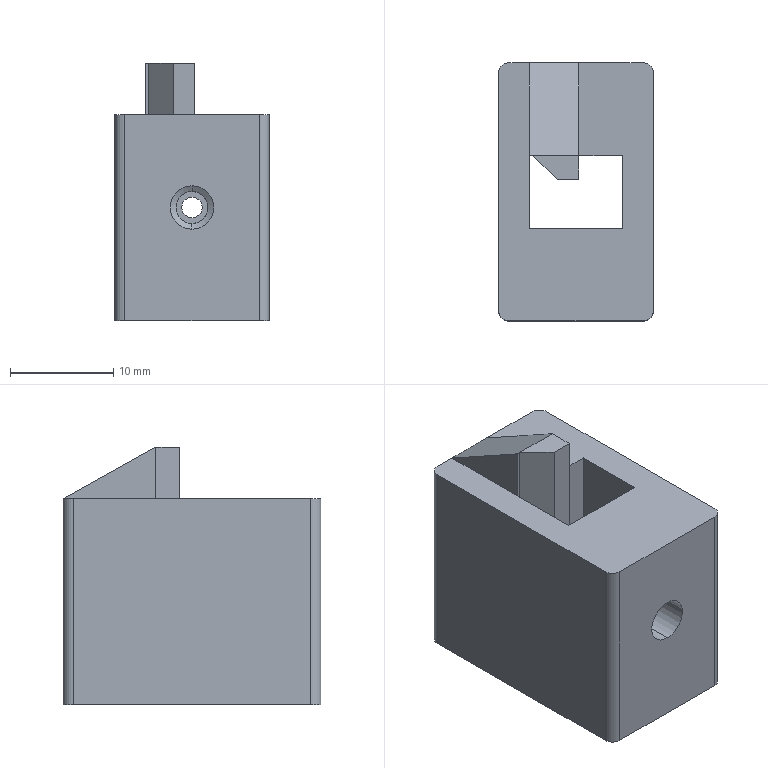Part | STEP file | 03-06 right pre-press cutter plate | 1 solid | 39 faces | box 15 x 25 x 25 mm | volume 5962 mm3 | plane 21 | cylinder 16 | cone 2 | commonest cylinder face diameters 2 x6 3.1 x4 7 x4 4.2 x2
STEP:
#1=CARTESIAN_POINT('',(0.,9.5,12.));
#2=VERTEX_POINT('',#1);
#3=CARTESIAN_POINT('',(0.,9.5,10.));
#4=VERTEX_POINT('',#3);
#5=CARTESIAN_POINT('',(0.,9.5,11.));
#6=DIRECTION('',(0.,-1.,0.));
#7=DIRECTION('',(0.,0.,-1.));
#8=AXIS2_PLACEMENT_3D('',#5,#6,#7);
#9=CIRCLE('',#8,1.);
#10=EDGE_CURVE('',#2,#4,#9,.T.);
#11=ORIENTED_EDGE('',*,*,#10,.T.);
#12=CARTESIAN_POINT('',(0.,12.5,10.));
#13=VERTEX_POINT('',#12);
#14=CARTESIAN_POINT('',(0.,2.5,10.));
#15=DIRECTION('',(0.,1.,0.));
#16=VECTOR('',#15,1000.);
#17=LINE('',#14,#16);
#18=EDGE_CURVE('',#4,#13,#17,.T.);
#19=ORIENTED_EDGE('',*,*,#18,.T.);
#20=CARTESIAN_POINT('',(0.,12.5,12.));
#21=VERTEX_POINT('',#20);
#22=CARTESIAN_POINT('',(0.,12.5,11.));
#23=DIRECTION('',(0.,1.,0.));
#24=DIRECTION('',(0.,0.,1.));
#25=AXIS2_PLACEMENT_3D('',#22,#23,#24);
#26=CIRCLE('',#25,1.);
#27=EDGE_CURVE('',#13,#21,#26,.T.);
#28=ORIENTED_EDGE('',*,*,#27,.T.);
#29=CARTESIAN_POINT('',(0.,2.5,12.));
#30=DIRECTION('',(0.,1.,0.));
#31=VECTOR('',#30,1000.);
#32=LINE('',#29,#31);
#33=EDGE_CURVE('',#2,#21,#32,.T.);
#34=ORIENTED_EDGE('',*,*,#33,.F.);
#35=EDGE_LOOP('',(#11,#19,#28,#34));
#36=FACE_OUTER_BOUND('',#35,.T.);
#37=CARTESIAN_POINT('',(0.,2.5,11.));
#38=DIRECTION('',(0.,1.,0.));
#39=DIRECTION('',(0.,0.,1.));
#40=AXIS2_PLACEMENT_3D('',#37,#38,#39);
#41=CYLINDRICAL_SURFACE('',#40,1.);
#42=ADVANCED_FACE('',(#36),#41,.F.);
#43=CARTESIAN_POINT('',(0.,-7.5,13.1));
#44=VERTEX_POINT('',#43);
#45=CARTESIAN_POINT('',(0.,-7.5,8.9));
#46=VERTEX_POINT('',#45);
#47=CARTESIAN_POINT('',(0.,-7.5,11.));
#48=DIRECTION('',(0.,-1.,0.));
#49=DIRECTION('',(0.,0.,-1.));
#50=AXIS2_PLACEMENT_3D('',#47,#48,#49);
#51=CIRCLE('',#50,2.1);
#52=EDGE_CURVE('',#44,#46,#51,.T.);
#53=ORIENTED_EDGE('',*,*,#52,.F.);
#54=CARTESIAN_POINT('',(0.,-12.5,13.1));
#55=VERTEX_POINT('',#54);
#56=CARTESIAN_POINT('',(0.,-12.5,13.1));
#57=DIRECTION('',(0.,-1.,0.));
#58=VECTOR('',#57,1000.);
#59=LINE('',#56,#58);
#60=EDGE_CURVE('',#44,#55,#59,.T.);
#61=ORIENTED_EDGE('',*,*,#60,.T.);
#62=CARTESIAN_POINT('',(0.,-12.5,8.9));
#63=VERTEX_POINT('',#62);
#64=CARTESIAN_POINT('',(0.,-12.5,11.));
#65=DIRECTION('',(0.,-1.,0.));
#66=DIRECTION('',(0.,0.,-1.));
#67=AXIS2_PLACEMENT_3D('',#64,#65,#66);
#68=CIRCLE('',#67,2.1);
#69=EDGE_CURVE('',#55,#63,#68,.T.);
#70=ORIENTED_EDGE('',*,*,#69,.T.);
#71=CARTESIAN_POINT('',(0.,-12.5,8.9));
#72=DIRECTION('',(0.,-1.,0.));
#73=VECTOR('',#72,1000.);
#74=LINE('',#71,#73);
#75=EDGE_CURVE('',#46,#63,#74,.T.);
#76=ORIENTED_EDGE('',*,*,#75,.F.);
#77=EDGE_LOOP('',(#53,#61,#70,#76));
#78=FACE_OUTER_BOUND('',#77,.T.);
#79=CARTESIAN_POINT('',(0.,-12.5,11.));
#80=DIRECTION('',(0.,-1.,0.));
#81=DIRECTION('',(0.,0.,-1.));
#82=AXIS2_PLACEMENT_3D('',#79,#80,#81);
#83=CYLINDRICAL_SURFACE('',#82,2.1);
#84=ADVANCED_FACE('',(#78),#83,.F.);
#85=CARTESIAN_POINT('',(0.,-7.17,12.55));
#86=VERTEX_POINT('',#85);
#87=CARTESIAN_POINT('',(0.,-7.17,9.45));
#88=VERTEX_POINT('',#87);
#89=CARTESIAN_POINT('',(0.,-7.17,11.));
#90=DIRECTION('',(0.,-1.,0.));
#91=DIRECTION('',(0.,0.,-1.));
#92=AXIS2_PLACEMENT_3D('',#89,#90,#91);
#93=CIRCLE('',#92,1.55);
#94=EDGE_CURVE('',#86,#88,#93,.T.);
#95=ORIENTED_EDGE('',*,*,#94,.F.);
#96=CARTESIAN_POINT('',(0.,-7.5,13.1));
#97=DIRECTION('',(0.,-0.515,0.8572));
#98=VECTOR('',#97,1000.);
#99=LINE('',#96,#98);
#100=EDGE_CURVE('',#86,#44,#99,.T.);
#101=ORIENTED_EDGE('',*,*,#100,.T.);
#102=ORIENTED_EDGE('',*,*,#52,.T.);
#103=CARTESIAN_POINT('',(0.,-7.5,8.9));
#104=DIRECTION('',(0.,-0.515,-0.8572));
#105=VECTOR('',#104,1000.);
#106=LINE('',#103,#105);
#107=EDGE_CURVE('',#88,#46,#106,.T.);
#108=ORIENTED_EDGE('',*,*,#107,.F.);
#109=EDGE_LOOP('',(#95,#101,#102,#108));
#110=FACE_OUTER_BOUND('',#109,.T.);
#111=CARTESIAN_POINT('',(0.,-7.5,11.));
#112=DIRECTION('',(0.,-1.,0.));
#113=DIRECTION('',(0.,0.,-1.));
#114=AXIS2_PLACEMENT_3D('',#111,#112,#113);
#115=CONICAL_SURFACE('',#114,2.1,1.03);
#116=ADVANCED_FACE('',(#110),#115,.F.);
#117=CARTESIAN_POINT('',(0.,-3.51,12.55));
#118=VERTEX_POINT('',#117);
#119=CARTESIAN_POINT('',(0.,-3.51,9.45));
#120=VERTEX_POINT('',#119);
#121=CARTESIAN_POINT('',(0.,-3.51,11.));
#122=DIRECTION('',(0.,-1.,0.));
#123=DIRECTION('',(1.,0.,0.));
#124=AXIS2_PLACEMENT_3D('',#121,#122,#123);
#125=CIRCLE('',#124,1.55);
#126=EDGE_CURVE('',#118,#120,#125,.T.);
#127=ORIENTED_EDGE('',*,*,#126,.F.);
#128=CARTESIAN_POINT('',(0.,9.5,12.55));
#129=DIRECTION('',(0.,-1.,0.));
#130=VECTOR('',#129,1000.);
#131=LINE('',#128,#130);
#132=EDGE_CURVE('',#118,#86,#131,.T.);
#133=ORIENTED_EDGE('',*,*,#132,.T.);
#134=ORIENTED_EDGE('',*,*,#94,.T.);
#135=CARTESIAN_POINT('',(0.,9.5,9.45));
#136=DIRECTION('',(0.,-1.,0.));
#137=VECTOR('',#136,1000.);
#138=LINE('',#135,#137);
#139=EDGE_CURVE('',#120,#88,#138,.T.);
#140=ORIENTED_EDGE('',*,*,#139,.F.);
#141=EDGE_LOOP('',(#127,#133,#134,#140));
#142=FACE_OUTER_BOUND('',#141,.T.);
#143=CARTESIAN_POINT('',(0.,9.5,11.));
#144=DIRECTION('',(0.,-1.,0.));
#145=DIRECTION('',(0.,0.,-1.));
#146=AXIS2_PLACEMENT_3D('',#143,#144,#145);
#147=CYLINDRICAL_SURFACE('',#146,1.55);
#148=ADVANCED_FACE('',(#142),#147,.F.);
#149=CARTESIAN_POINT('',(0.,9.5,12.55));
#150=VERTEX_POINT('',#149);
#151=CARTESIAN_POINT('',(0.,9.5,9.45));
#152=VERTEX_POINT('',#151);
#153=CARTESIAN_POINT('',(0.,9.5,11.));
#154=DIRECTION('',(0.,-1.,0.));
#155=DIRECTION('',(0.,0.,-1.));
#156=AXIS2_PLACEMENT_3D('',#153,#154,#155);
#157=CIRCLE('',#156,1.55);
#158=EDGE_CURVE('',#150,#152,#157,.T.);
#159=ORIENTED_EDGE('',*,*,#158,.F.);
#160=CARTESIAN_POINT('',(0.,1.199,12.55));
#161=VERTEX_POINT('',#160);
#162=CARTESIAN_POINT('',(0.,9.5,12.55));
#163=DIRECTION('',(0.,-1.,0.));
#164=VECTOR('',#163,1000.);
#165=LINE('',#162,#164);
#166=EDGE_CURVE('',#150,#161,#165,.T.);
#167=ORIENTED_EDGE('',*,*,#166,.T.);
#168=CARTESIAN_POINT('',(0.,1.199,9.45));
#169=VERTEX_POINT('',#168);
#170=CARTESIAN_POINT('',(0.,1.199,11.));
#171=DIRECTION('',(0.,1.,0.));
#172=DIRECTION('',(0.,0.,1.));
#173=AXIS2_PLACEMENT_3D('',#170,#171,#172);
#174=CIRCLE('',#173,1.55);
#175=EDGE_CURVE('',#169,#161,#174,.T.);
#176=ORIENTED_EDGE('',*,*,#175,.F.);
#177=CARTESIAN_POINT('',(0.,9.5,9.45));
#178=DIRECTION('',(0.,-1.,0.));
#179=VECTOR('',#178,1000.);
#180=LINE('',#177,#179);
#181=EDGE_CURVE('',#152,#169,#180,.T.);
#182=ORIENTED_EDGE('',*,*,#181,.F.);
#183=EDGE_LOOP('',(#159,#167,#176,#182));
#184=FACE_OUTER_BOUND('',#183,.T.);
#185=CARTESIAN_POINT('',(0.,9.5,11.));
#186=DIRECTION('',(0.,-1.,0.));
#187=DIRECTION('',(0.,0.,-1.));
#188=AXIS2_PLACEMENT_3D('',#185,#186,#187);
#189=CYLINDRICAL_SURFACE('',#188,1.55);
#190=ADVANCED_FACE('',(#184),#189,.F.);
#191=CARTESIAN_POINT('',(3.5,-8.,5.));
#192=VERTEX_POINT('',#191);
#193=CARTESIAN_POINT('',(-3.5,-8.,5.));
#194=VERTEX_POINT('',#193);
#195=CARTESIAN_POINT('',(0.,-8.,5.));
#196=DIRECTION('',(0.,0.,-1.));
#197=DIRECTION('',(-1.,0.,0.));
#198=AXIS2_PLACEMENT_3D('',#195,#196,#197);
#199=CIRCLE('',#198,3.5);
#200=EDGE_CURVE('',#192,#194,#199,.T.);
#201=ORIENTED_EDGE('',*,*,#200,.F.);
#202=CARTESIAN_POINT('',(3.5,-8.,0.));
#203=VERTEX_POINT('',#202);
#204=CARTESIAN_POINT('',(3.5,-8.,5.));
#205=DIRECTION('',(0.,0.,-1.));
#206=VECTOR('',#205,1000.);
#207=LINE('',#204,#206);
#208=EDGE_CURVE('',#192,#203,#207,.T.);
#209=ORIENTED_EDGE('',*,*,#208,.T.);
#210=CARTESIAN_POINT('',(-3.5,-8.,0.));
#211=VERTEX_POINT('',#210);
#212=CARTESIAN_POINT('',(0.,-8.,0.));
#213=DIRECTION('',(0.,0.,-1.));
#214=DIRECTION('',(-1.,0.,0.));
#215=AXIS2_PLACEMENT_3D('',#212,#213,#214);
#216=CIRCLE('',#215,3.5);
#217=EDGE_CURVE('',#203,#211,#216,.T.);
#218=ORIENTED_EDGE('',*,*,#217,.T.);
#219=CARTESIAN_POINT('',(-3.5,-8.,5.));
#220=DIRECTION('',(0.,0.,-1.));
#221=VECTOR('',#220,1000.);
#222=LINE('',#219,#221);
#223=EDGE_CURVE('',#194,#211,#222,.T.);
#224=ORIENTED_EDGE('',*,*,#223,.F.);
#225=EDGE_LOOP('',(#201,#209,#218,#224));
#226=FACE_OUTER_BOUND('',#225,.T.);
#227=CARTESIAN_POINT('',(0.,-8.,5.));
#228=DIRECTION('',(0.,0.,-1.));
#229=DIRECTION('',(-1.,0.,0.));
#230=AXIS2_PLACEMENT_3D('',#227,#228,#229);
#231=CYLINDRICAL_SURFACE('',#230,3.5);
#232=ADVANCED_FACE('',(#226),#231,.F.);
#233=CARTESIAN_POINT('',(3.5,8.,5.));
#234=VERTEX_POINT('',#233);
#235=CARTESIAN_POINT('',(-3.5,8.,5.));
#236=VERTEX_POINT('',#235);
#237=CARTESIAN_POINT('',(0.,8.,5.));
#238=DIRECTION('',(0.,0.,-1.));
#239=DIRECTION('',(-1.,0.,0.));
#240=AXIS2_PLACEMENT_3D('',#237,#238,#239);
#241=CIRCLE('',#240,3.5);
#242=EDGE_CURVE('',#234,#236,#241,.T.);
#243=ORIENTED_EDGE('',*,*,#242,.F.);
#244=CARTESIAN_POINT('',(3.5,8.,0.));
#245=VERTEX_POINT('',#244);
#246=CARTESIAN_POINT('',(3.5,8.,5.));
#247=DIRECTION('',(0.,0.,-1.));
#248=VECTOR('',#247,1000.);
#249=LINE('',#246,#248);
#250=EDGE_CURVE('',#234,#245,#249,.T.);
#251=ORIENTED_EDGE('',*,*,#250,.T.);
#252=CARTESIAN_POINT('',(-3.5,8.,0.));
#253=VERTEX_POINT('',#252);
#254=CARTESIAN_POINT('',(0.,8.,0.));
#255=DIRECTION('',(0.,0.,-1.));
#256=DIRECTION('',(-1.,0.,0.));
#257=AXIS2_PLACEMENT_3D('',#254,#255,#256);
#258=CIRCLE('',#257,3.5);
#259=EDGE_CURVE('',#245,#253,#258,.T.);
#260=ORIENTED_EDGE('',*,*,#259,.T.);
#261=CARTESIAN_POINT('',(-3.5,8.,5.));
#262=DIRECTION('',(0.,0.,-1.));
#263=VECTOR('',#262,1000.);
#264=LINE('',#261,#263);
#265=EDGE_CURVE('',#236,#253,#264,.T.);
#266=ORIENTED_EDGE('',*,*,#265,.F.);
#267=EDGE_LOOP('',(#243,#251,#260,#266));
#268=FACE_OUTER_BOUND('',#267,.T.);
#269=CARTESIAN_POINT('',(0.,8.,5.));
#270=DIRECTION('',(0.,0.,-1.));
#271=DIRECTION('',(-1.,0.,0.));
#272=AXIS2_PLACEMENT_3D('',#269,#270,#271);
#273=CYLINDRICAL_SURFACE('',#272,3.5);
#274=ADVANCED_FACE('',(#268),#273,.F.);
#275=CARTESIAN_POINT('',(0.2629,3.51,0.));
#276=VERTEX_POINT('',#275);
#277=CARTESIAN_POINT('',(0.2629,3.51,9.472));
#278=VERTEX_POINT('',#277);
#279=CARTESIAN_POINT('',(0.2629,3.51,-2.));
#280=DIRECTION('',(0.,0.,1.));
#281=VECTOR('',#280,1000.);
#282=LINE('',#279,#281);
#283=EDGE_CURVE('',#276,#278,#282,.T.);
#284=ORIENTED_EDGE('',*,*,#283,.T.);
#285=CARTESIAN_POINT('',(0.2629,1.199,9.472));
#286=VERTEX_POINT('',#285);
#287=CARTESIAN_POINT('',(0.2629,9.5,9.472));
#288=DIRECTION('',(0.,-1.,0.));
#289=VECTOR('',#288,1000.);
#290=LINE('',#287,#289);
#291=EDGE_CURVE('',#278,#286,#290,.T.);
#292=ORIENTED_EDGE('',*,*,#291,.T.);
#293=CARTESIAN_POINT('',(0.2629,1.199,0.));
#294=VERTEX_POINT('',#293);
#295=CARTESIAN_POINT('',(0.2629,1.199,-2.));
#296=DIRECTION('',(0.,0.,1.));
#297=VECTOR('',#296,1000.);
#298=LINE('',#295,#297);
#299=EDGE_CURVE('',#294,#286,#298,.T.);
#300=ORIENTED_EDGE('',*,*,#299,.F.);
#301=CARTESIAN_POINT('',(0.2629,-12.5,0.));
#302=DIRECTION('',(0.,-1.,0.));
#303=VECTOR('',#302,1000.);
#304=LINE('',#301,#303);
#305=EDGE_CURVE('',#276,#294,#304,.T.);
#306=ORIENTED_EDGE('',*,*,#305,.F.);
#307=EDGE_LOOP('',(#284,#292,#300,#306));
#308=FACE_OUTER_BOUND('',#307,.T.);
#309=CARTESIAN_POINT('',(0.2629,1.199,-2.));
#310=DIRECTION('',(-1.,0.,0.));
#311=DIRECTION('',(0.,-1.,0.));
#312=AXIS2_PLACEMENT_3D('',#309,#310,#311);
#313=PLANE('',#312);
#314=ADVANCED_FACE('',(#308),#313,.F.);
#315=CARTESIAN_POINT('',(7.5,-11.5,20.));
#316=VERTEX_POINT('',#315);
#317=CARTESIAN_POINT('',(7.5,11.5,20.));
#318=VERTEX_POINT('',#317);
#319=CARTESIAN_POINT('',(7.5,12.5,20.));
#320=DIRECTION('',(0.,1.,0.));
#321=VECTOR('',#320,1000.);
#322=LINE('',#319,#321);
#323=EDGE_CURVE('',#316,#318,#322,.T.);
#324=ORIENTED_EDGE('',*,*,#323,.F.);
#325=CARTESIAN_POINT('',(7.5,-11.5,0.));
#326=VERTEX_POINT('',#325);
#327=CARTESIAN_POINT('',(7.5,-11.5,25.));
#328=DIRECTION('',(0.,0.,-1.));
#329=VECTOR('',#328,1000.);
#330=LINE('',#327,#329);
#331=EDGE_CURVE('',#316,#326,#330,.T.);
#332=ORIENTED_EDGE('',*,*,#331,.T.);
#333=CARTESIAN_POINT('',(7.5,11.5,0.));
#334=VERTEX_POINT('',#333);
#335=CARTESIAN_POINT('',(7.5,12.5,0.));
#336=DIRECTION('',(0.,1.,0.));
#337=VECTOR('',#336,1000.);
#338=LINE('',#335,#337);
#339=EDGE_CURVE('',#326,#334,#338,.T.);
#340=ORIENTED_EDGE('',*,*,#339,.T.);
#341=CARTESIAN_POINT('',(7.5,11.5,25.));
#342=DIRECTION('',(0.,0.,1.));
#343=VECTOR('',#342,1000.);
#344=LINE('',#341,#343);
#345=EDGE_CURVE('',#334,#318,#344,.T.);
#346=ORIENTED_EDGE('',*,*,#345,.T.);
#347=EDGE_LOOP('',(#324,#332,#340,#346));
#348=FACE_OUTER_BOUND('',#347,.T.);
#349=CARTESIAN_POINT('',(7.5,12.5,25.));
#350=DIRECTION('',(-1.,0.,0.));
#351=DIRECTION('',(0.,-1.,0.));
#352=AXIS2_PLACEMENT_3D('',#349,#350,#351);
#353=PLANE('',#352);
#354=ADVANCED_FACE('',(#348),#353,.F.);
#355=CARTESIAN_POINT('',(0.,12.5,11.));
#356=DIRECTION('',(0.,1.,0.));
#357=DIRECTION('',(0.,0.,1.));
#358=AXIS2_PLACEMENT_3D('',#355,#356,#357);
#359=CIRCLE('',#358,1.);
#360=EDGE_CURVE('',#21,#13,#359,.T.);
#361=ORIENTED_EDGE('',*,*,#360,.F.);
#362=ORIENTED_EDGE('',*,*,#27,.F.);
#363=EDGE_LOOP('',(#361,#362));
#364=FACE_BOUND('',#363,.T.);
#365=CARTESIAN_POINT('',(6.5,12.5,0.));
#366=VERTEX_POINT('',#365);
#367=CARTESIAN_POINT('',(-6.5,12.5,0.));
#368=VERTEX_POINT('',#367);
#369=CARTESIAN_POINT('',(-7.5,12.5,0.));
#370=DIRECTION('',(-1.,0.,0.));
#371=VECTOR('',#370,1000.);
#372=LINE('',#369,#371);
#373=EDGE_CURVE('',#366,#368,#372,.T.);
#374=ORIENTED_EDGE('',*,*,#373,.T.);
#375=CARTESIAN_POINT('',(-6.5,12.5,20.));
#376=VERTEX_POINT('',#375);
#377=CARTESIAN_POINT('',(-6.5,12.5,25.));
#378=DIRECTION('',(0.,0.,1.));
#379=VECTOR('',#378,1000.);
#380=LINE('',#377,#379);
#381=EDGE_CURVE('',#368,#376,#380,.T.);
#382=ORIENTED_EDGE('',*,*,#381,.T.);
#383=CARTESIAN_POINT('',(-4.51,12.5,20.));
#384=VERTEX_POINT('',#383);
#385=CARTESIAN_POINT('',(-17.787,12.5,20.));
#386=DIRECTION('',(1.,0.,0.));
#387=VECTOR('',#386,1000.);
#388=LINE('',#385,#387);
#389=EDGE_CURVE('',#376,#384,#388,.T.);
#390=ORIENTED_EDGE('',*,*,#389,.T.);
#391=CARTESIAN_POINT('',(0.2629,12.5,20.));
#392=VERTEX_POINT('',#391);
#393=CARTESIAN_POINT('',(-17.787,12.5,20.));
#394=DIRECTION('',(1.,0.,0.));
#395=VECTOR('',#394,1000.);
#396=LINE('',#393,#395);
#397=EDGE_CURVE('',#384,#392,#396,.T.);
#398=ORIENTED_EDGE('',*,*,#397,.T.);
#399=CARTESIAN_POINT('',(6.5,12.5,20.));
#400=VERTEX_POINT('',#399);
#401=CARTESIAN_POINT('',(-7.5,12.5,20.));
#402=DIRECTION('',(-1.,0.,0.));
#403=VECTOR('',#402,1000.);
#404=LINE('',#401,#403);
#405=EDGE_CURVE('',#400,#392,#404,.T.);
#406=ORIENTED_EDGE('',*,*,#405,.F.);
#407=CARTESIAN_POINT('',(6.5,12.5,25.));
#408=DIRECTION('',(0.,0.,-1.));
#409=VECTOR('',#408,1000.);
#410=LINE('',#407,#409);
#411=EDGE_CURVE('',#400,#366,#410,.T.);
#412=ORIENTED_EDGE('',*,*,#411,.T.);
#413=EDGE_LOOP('',(#374,#382,#390,#398,#406,#412));
#414=FACE_OUTER_BOUND('',#413,.T.);
#415=CARTESIAN_POINT('',(-7.5,12.5,25.));
#416=DIRECTION('',(0.,-1.,0.));
#417=DIRECTION('',(0.,0.,-1.));
#418=AXIS2_PLACEMENT_3D('',#415,#416,#417);
#419=PLANE('',#418);
#420=ADVANCED_FACE('',(#364,#414),#419,.F.);
#421=CARTESIAN_POINT('',(-7.5,11.5,20.));
#422=VERTEX_POINT('',#421);
#423=CARTESIAN_POINT('',(-7.5,-11.5,20.));
#424=VERTEX_POINT('',#423);
#425=CARTESIAN_POINT('',(-7.5,12.5,20.));
#426=DIRECTION('',(0.,-1.,0.));
#427=VECTOR('',#426,1000.);
#428=LINE('',#425,#427);
#429=EDGE_CURVE('',#422,#424,#428,.T.);
#430=ORIENTED_EDGE('',*,*,#429,.F.);
#431=CARTESIAN_POINT('',(-7.5,11.5,0.));
#432=VERTEX_POINT('',#431);
#433=CARTESIAN_POINT('',(-7.5,11.5,25.));
#434=DIRECTION('',(0.,0.,-1.));
#435=VECTOR('',#434,1000.);
#436=LINE('',#433,#435);
#437=EDGE_CURVE('',#422,#432,#436,.T.);
#438=ORIENTED_EDGE('',*,*,#437,.T.);
#439=CARTESIAN_POINT('',(-7.5,-11.5,0.));
#440=VERTEX_POINT('',#439);
#441=CARTESIAN_POINT('',(-7.5,12.5,0.));
#442=DIRECTION('',(0.,-1.,0.));
#443=VECTOR('',#442,1000.);
#444=LINE('',#441,#443);
#445=EDGE_CURVE('',#432,#440,#444,.T.);
#446=ORIENTED_EDGE('',*,*,#445,.T.);
#447=CARTESIAN_POINT('',(-7.5,-11.5,25.));
#448=DIRECTION('',(0.,0.,1.));
#449=VECTOR('',#448,1000.);
#450=LINE('',#447,#449);
#451=EDGE_CURVE('',#440,#424,#450,.T.);
#452=ORIENTED_EDGE('',*,*,#451,.T.);
#453=EDGE_LOOP('',(#430,#438,#446,#452));
#454=FACE_OUTER_BOUND('',#453,.T.);
#455=CARTESIAN_POINT('',(-7.5,12.5,25.));
#456=DIRECTION('',(1.,0.,0.));
#457=DIRECTION('',(0.,1.,0.));
#458=AXIS2_PLACEMENT_3D('',#455,#456,#457);
#459=PLANE('',#458);
#460=ADVANCED_FACE('',(#454),#459,.F.);
#461=CARTESIAN_POINT('',(0.,-12.5,11.));
#462=DIRECTION('',(0.,-1.,0.));
#463=DIRECTION('',(0.,0.,-1.));
#464=AXIS2_PLACEMENT_3D('',#461,#462,#463);
#465=CIRCLE('',#464,2.1);
#466=EDGE_CURVE('',#63,#55,#465,.T.);
#467=ORIENTED_EDGE('',*,*,#466,.F.);
#468=ORIENTED_EDGE('',*,*,#69,.F.);
#469=EDGE_LOOP('',(#467,#468));
#470=FACE_BOUND('',#469,.T.);
#471=CARTESIAN_POINT('',(-6.5,-12.5,20.));
#472=VERTEX_POINT('',#471);
#473=CARTESIAN_POINT('',(6.5,-12.5,20.));
#474=VERTEX_POINT('',#473);
#475=CARTESIAN_POINT('',(-7.5,-12.5,20.));
#476=DIRECTION('',(1.,0.,0.));
#477=VECTOR('',#476,1000.);
#478=LINE('',#475,#477);
#479=EDGE_CURVE('',#472,#474,#478,.T.);
#480=ORIENTED_EDGE('',*,*,#479,.F.);
#481=CARTESIAN_POINT('',(-6.5,-12.5,0.));
#482=VERTEX_POINT('',#481);
#483=CARTESIAN_POINT('',(-6.5,-12.5,25.));
#484=DIRECTION('',(0.,0.,-1.));
#485=VECTOR('',#484,1000.);
#486=LINE('',#483,#485);
#487=EDGE_CURVE('',#472,#482,#486,.T.);
#488=ORIENTED_EDGE('',*,*,#487,.T.);
#489=CARTESIAN_POINT('',(6.5,-12.5,0.));
#490=VERTEX_POINT('',#489);
#491=CARTESIAN_POINT('',(-7.5,-12.5,0.));
#492=DIRECTION('',(1.,0.,0.));
#493=VECTOR('',#492,1000.);
#494=LINE('',#491,#493);
#495=EDGE_CURVE('',#482,#490,#494,.T.);
#496=ORIENTED_EDGE('',*,*,#495,.T.);
#497=CARTESIAN_POINT('',(6.5,-12.5,25.));
#498=DIRECTION('',(0.,0.,1.));
#499=VECTOR('',#498,1000.);
#500=LINE('',#497,#499);
#501=EDGE_CURVE('',#490,#474,#500,.T.);
#502=ORIENTED_EDGE('',*,*,#501,.T.);
#503=EDGE_LOOP('',(#480,#488,#496,#502));
#504=FACE_OUTER_BOUND('',#503,.T.);
#505=CARTESIAN_POINT('',(-7.5,-12.5,25.));
#506=DIRECTION('',(0.,1.,0.));
#507=DIRECTION('',(0.,0.,1.));
#508=AXIS2_PLACEMENT_3D('',#505,#506,#507);
#509=PLANE('',#508);
#510=ADVANCED_FACE('',(#470,#504),#509,.F.);
#511=CARTESIAN_POINT('',(0.2629,3.51,25.));
#512=VERTEX_POINT('',#511);
#513=CARTESIAN_POINT('',(0.2629,1.199,25.));
#514=VERTEX_POINT('',#513);
#515=CARTESIAN_POINT('',(0.2629,1.199,25.));
#516=DIRECTION('',(0.,-1.,0.));
#517=VECTOR('',#516,1000.);
#518=LINE('',#515,#517);
#519=EDGE_CURVE('',#512,#514,#518,.T.);
#520=ORIENTED_EDGE('',*,*,#519,.F.);
#521=CARTESIAN_POINT('',(-4.198,3.51,25.));
#522=VERTEX_POINT('',#521);
#523=CARTESIAN_POINT('',(-4.51,3.51,25.));
#524=DIRECTION('',(-1.,0.,0.));
#525=VECTOR('',#524,1000.);
#526=LINE('',#523,#525);
#527=EDGE_CURVE('',#512,#522,#526,.T.);
#528=ORIENTED_EDGE('',*,*,#527,.T.);
#529=CARTESIAN_POINT('',(-1.809,1.199,25.));
#530=VERTEX_POINT('',#529);
#531=CARTESIAN_POINT('',(-1.809,1.199,25.));
#532=DIRECTION('',(-0.7187,0.6953,0.));
#533=VECTOR('',#532,1000.);
#534=LINE('',#531,#533);
#535=EDGE_CURVE('',#530,#522,#534,.T.);
#536=ORIENTED_EDGE('',*,*,#535,.F.);
#537=CARTESIAN_POINT('',(-1.809,1.199,25.));
#538=DIRECTION('',(-1.,0.,0.));
#539=VECTOR('',#538,1000.);
#540=LINE('',#537,#539);
#541=EDGE_CURVE('',#514,#530,#540,.T.);
#542=ORIENTED_EDGE('',*,*,#541,.F.);
#543=EDGE_LOOP('',(#520,#528,#536,#542));
#544=FACE_OUTER_BOUND('',#543,.T.);
#545=CARTESIAN_POINT('',(7.5,-12.5,25.));
#546=DIRECTION('',(0.,0.,1.));
#547=DIRECTION('',(1.,0.,0.));
#548=AXIS2_PLACEMENT_3D('',#545,#546,#547);
#549=PLANE('',#548);
#550=ADVANCED_FACE('',(#544),#549,.T.);
#551=CARTESIAN_POINT('',(4.51,-3.51,20.));
#552=VERTEX_POINT('',#551);
#553=CARTESIAN_POINT('',(4.51,3.51,20.));
#554=VERTEX_POINT('',#553);
#555=CARTESIAN_POINT('',(4.51,3.51,20.));
#556=DIRECTION('',(0.,1.,0.));
#557=VECTOR('',#556,1000.);
#558=LINE('',#555,#557);
#559=EDGE_CURVE('',#552,#554,#558,.T.);
#560=ORIENTED_EDGE('',*,*,#559,.T.);
#561=CARTESIAN_POINT('',(4.51,3.51,0.));
#562=VERTEX_POINT('',#561);
#563=CARTESIAN_POINT('',(4.51,3.51,-2.));
#564=DIRECTION('',(0.,0.,1.));
#565=VECTOR('',#564,1000.);
#566=LINE('',#563,#565);
#567=EDGE_CURVE('',#562,#554,#566,.T.);
#568=ORIENTED_EDGE('',*,*,#567,.F.);
#569=CARTESIAN_POINT('',(4.51,-3.51,0.));
#570=VERTEX_POINT('',#569);
#571=CARTESIAN_POINT('',(4.51,-12.5,0.));
#572=DIRECTION('',(0.,1.,0.));
#573=VECTOR('',#572,1000.);
#574=LINE('',#571,#573);
#575=EDGE_CURVE('',#570,#562,#574,.T.);
#576=ORIENTED_EDGE('',*,*,#575,.F.);
#577=CARTESIAN_POINT('',(4.51,-3.51,-2.));
#578=DIRECTION('',(0.,0.,1.));
#579=VECTOR('',#578,1000.);
#580=LINE('',#577,#579);
#581=EDGE_CURVE('',#570,#552,#580,.T.);
#582=ORIENTED_EDGE('',*,*,#581,.T.);
#583=EDGE_LOOP('',(#560,#568,#576,#582));
#584=FACE_OUTER_BOUND('',#583,.T.);
#585=CARTESIAN_POINT('',(4.51,3.51,-2.));
#586=DIRECTION('',(1.,0.,0.));
#587=DIRECTION('',(0.,0.,-1.));
#588=AXIS2_PLACEMENT_3D('',#585,#586,#587);
#589=PLANE('',#588);
#590=ADVANCED_FACE('',(#584),#589,.F.);
#591=CARTESIAN_POINT('',(0.,-3.51,11.));
#592=DIRECTION('',(0.,-1.,0.));
#593=DIRECTION('',(1.,0.,0.));
#594=AXIS2_PLACEMENT_3D('',#591,#592,#593);
#595=CIRCLE('',#594,1.55);
#596=EDGE_CURVE('',#120,#118,#595,.T.);
#597=ORIENTED_EDGE('',*,*,#596,.T.);
#598=ORIENTED_EDGE('',*,*,#126,.T.);
#599=EDGE_LOOP('',(#597,#598));
#600=FACE_BOUND('',#599,.T.);
#601=CARTESIAN_POINT('',(-4.51,-3.51,20.));
#602=VERTEX_POINT('',#601);
#603=CARTESIAN_POINT('',(-4.51,-3.51,20.));
#604=DIRECTION('',(1.,0.,0.));
#605=VECTOR('',#604,1000.);
#606=LINE('',#603,#605);
#607=EDGE_CURVE('',#602,#552,#606,.T.);
#608=ORIENTED_EDGE('',*,*,#607,.T.);
#609=ORIENTED_EDGE('',*,*,#581,.F.);
#610=CARTESIAN_POINT('',(-4.51,-3.51,0.));
#611=VERTEX_POINT('',#610);
#612=CARTESIAN_POINT('',(7.5,-3.51,0.));
#613=DIRECTION('',(1.,0.,0.));
#614=VECTOR('',#613,1000.);
#615=LINE('',#612,#614);
#616=EDGE_CURVE('',#611,#570,#615,.T.);
#617=ORIENTED_EDGE('',*,*,#616,.F.);
#618=CARTESIAN_POINT('',(-4.51,-3.51,-2.));
#619=DIRECTION('',(0.,0.,1.));
#620=VECTOR('',#619,1000.);
#621=LINE('',#618,#620);
#622=EDGE_CURVE('',#611,#602,#621,.T.);
#623=ORIENTED_EDGE('',*,*,#622,.T.);
#624=EDGE_LOOP('',(#608,#609,#617,#623));
#625=FACE_OUTER_BOUND('',#624,.T.);
#626=CARTESIAN_POINT('',(4.51,-3.51,-2.));
#627=DIRECTION('',(0.,-1.,0.));
#628=DIRECTION('',(1.,0.,0.));
#629=AXIS2_PLACEMENT_3D('',#626,#627,#628);
#630=PLANE('',#629);
#631=ADVANCED_FACE('',(#600,#625),#630,.F.);
#632=CARTESIAN_POINT('',(-4.51,3.51,20.));
#633=VERTEX_POINT('',#632);
#634=CARTESIAN_POINT('',(-4.51,3.51,20.));
#635=DIRECTION('',(0.,-1.,0.));
#636=VECTOR('',#635,1000.);
#637=LINE('',#634,#636);
#638=EDGE_CURVE('',#633,#602,#637,.T.);
#639=ORIENTED_EDGE('',*,*,#638,.T.);
#640=ORIENTED_EDGE('',*,*,#622,.F.);
#641=CARTESIAN_POINT('',(-4.51,3.51,0.));
#642=VERTEX_POINT('',#641);
#643=CARTESIAN_POINT('',(-4.51,-12.5,0.));
#644=DIRECTION('',(0.,-1.,0.));
#645=VECTOR('',#644,1000.);
#646=LINE('',#643,#645);
#647=EDGE_CURVE('',#642,#611,#646,.T.);
#648=ORIENTED_EDGE('',*,*,#647,.F.);
#649=CARTESIAN_POINT('',(-4.51,3.51,-2.));
#650=DIRECTION('',(0.,0.,1.));
#651=VECTOR('',#650,1000.);
#652=LINE('',#649,#651);
#653=EDGE_CURVE('',#642,#633,#652,.T.);
#654=ORIENTED_EDGE('',*,*,#653,.T.);
#655=EDGE_LOOP('',(#639,#640,#648,#654));
#656=FACE_OUTER_BOUND('',#655,.T.);
#657=CARTESIAN_POINT('',(-4.51,3.51,-2.));
#658=DIRECTION('',(-1.,0.,0.));
#659=DIRECTION('',(0.,-1.,0.));
#660=AXIS2_PLACEMENT_3D('',#657,#658,#659);
#661=PLANE('',#660);
#662=ADVANCED_FACE('',(#656),#661,.F.);
#663=CARTESIAN_POINT('',(-4.51,3.51,25.));
#664=VERTEX_POINT('',#663);
#665=CARTESIAN_POINT('',(-17.787,3.51,25.));
#666=DIRECTION('',(1.,0.,0.));
#667=VECTOR('',#666,1000.);
#668=LINE('',#665,#667);
#669=EDGE_CURVE('',#664,#522,#668,.T.);
#670=ORIENTED_EDGE('',*,*,#669,.F.);
#671=CARTESIAN_POINT('',(-4.51,3.51,25.));
#672=DIRECTION('',(0.,0.,1.));
#673=VECTOR('',#672,1000.);
#674=LINE('',#671,#673);
#675=EDGE_CURVE('',#633,#664,#674,.T.);
#676=ORIENTED_EDGE('',*,*,#675,.F.);
#677=ORIENTED_EDGE('',*,*,#653,.F.);
#678=CARTESIAN_POINT('',(-4.198,3.51,0.));
#679=VERTEX_POINT('',#678);
#680=CARTESIAN_POINT('',(7.5,3.51,0.));
#681=DIRECTION('',(-1.,0.,0.));
#682=VECTOR('',#681,1000.);
#683=LINE('',#680,#682);
#684=EDGE_CURVE('',#679,#642,#683,.T.);
#685=ORIENTED_EDGE('',*,*,#684,.F.);
#686=CARTESIAN_POINT('',(-4.198,3.51,-2.));
#687=DIRECTION('',(0.,0.,1.));
#688=VECTOR('',#687,1000.);
#689=LINE('',#686,#688);
#690=EDGE_CURVE('',#679,#522,#689,.T.);
#691=ORIENTED_EDGE('',*,*,#690,.T.);
#692=EDGE_LOOP('',(#670,#676,#677,#685,#691));
#693=FACE_OUTER_BOUND('',#692,.T.);
#694=CARTESIAN_POINT('',(-4.198,3.51,-2.));
#695=DIRECTION('',(0.,1.,0.));
#696=DIRECTION('',(-1.,0.,0.));
#697=AXIS2_PLACEMENT_3D('',#694,#695,#696);
#698=PLANE('',#697);
#699=ADVANCED_FACE('',(#693),#698,.F.);
#700=CARTESIAN_POINT('',(0.2629,3.51,12.528));
#701=VERTEX_POINT('',#700);
#702=CARTESIAN_POINT('',(0.2629,3.51,20.));
#703=VERTEX_POINT('',#702);
#704=CARTESIAN_POINT('',(0.2629,3.51,-2.));
#705=DIRECTION('',(0.,0.,1.));
#706=VECTOR('',#705,1000.);
#707=LINE('',#704,#706);
#708=EDGE_CURVE('',#701,#703,#707,.T.);
#709=ORIENTED_EDGE('',*,*,#708,.F.);
#710=CARTESIAN_POINT('',(0.,3.51,11.));
#711=DIRECTION('',(0.,1.,0.));
#712=DIRECTION('',(-1.,0.,0.));
#713=AXIS2_PLACEMENT_3D('',#710,#711,#712);
#714=CIRCLE('',#713,1.55);
#715=EDGE_CURVE('',#701,#278,#714,.T.);
#716=ORIENTED_EDGE('',*,*,#715,.T.);
#717=ORIENTED_EDGE('',*,*,#283,.F.);
#718=CARTESIAN_POINT('',(7.5,3.51,0.));
#719=DIRECTION('',(-1.,0.,0.));
#720=VECTOR('',#719,1000.);
#721=LINE('',#718,#720);
#722=EDGE_CURVE('',#562,#276,#721,.T.);
#723=ORIENTED_EDGE('',*,*,#722,.F.);
#724=ORIENTED_EDGE('',*,*,#567,.T.);
#725=CARTESIAN_POINT('',(-4.51,3.51,20.));
#726=DIRECTION('',(-1.,0.,0.));
#727=VECTOR('',#726,1000.);
#728=LINE('',#725,#727);
#729=EDGE_CURVE('',#554,#703,#728,.T.);
#730=ORIENTED_EDGE('',*,*,#729,.T.);
#731=EDGE_LOOP('',(#709,#716,#717,#723,#724,#730));
#732=FACE_OUTER_BOUND('',#731,.T.);
#733=CARTESIAN_POINT('',(4.51,3.51,-2.));
#734=DIRECTION('',(0.,1.,0.));
#735=DIRECTION('',(-1.,0.,0.));
#736=AXIS2_PLACEMENT_3D('',#733,#734,#735);
#737=PLANE('',#736);
#738=ADVANCED_FACE('',(#732),#737,.F.);
#739=CARTESIAN_POINT('',(0.,-8.,0.));
#740=DIRECTION('',(0.,0.,-1.));
#741=DIRECTION('',(-1.,0.,0.));
#742=AXIS2_PLACEMENT_3D('',#739,#740,#741);
#743=CIRCLE('',#742,3.5);
#744=EDGE_CURVE('',#211,#203,#743,.T.);
#745=ORIENTED_EDGE('',*,*,#744,.F.);
#746=ORIENTED_EDGE('',*,*,#217,.F.);
#747=EDGE_LOOP('',(#745,#746));
#748=FACE_BOUND('',#747,.T.);
#749=CARTESIAN_POINT('',(0.,8.,0.));
#750=DIRECTION('',(0.,0.,-1.));
#751=DIRECTION('',(-1.,0.,0.));
#752=AXIS2_PLACEMENT_3D('',#749,#750,#751);
#753=CIRCLE('',#752,3.5);
#754=EDGE_CURVE('',#253,#245,#753,.T.);
#755=ORIENTED_EDGE('',*,*,#754,.F.);
#756=ORIENTED_EDGE('',*,*,#259,.F.);
#757=EDGE_LOOP('',(#755,#756));
#758=FACE_BOUND('',#757,.T.);
#759=ORIENTED_EDGE('',*,*,#616,.T.);
#760=ORIENTED_EDGE('',*,*,#575,.T.);
#761=ORIENTED_EDGE('',*,*,#722,.T.);
#762=ORIENTED_EDGE('',*,*,#305,.T.);
#763=CARTESIAN_POINT('',(-1.809,1.199,0.));
#764=VERTEX_POINT('',#763);
#765=CARTESIAN_POINT('',(7.5,1.199,0.));
#766=DIRECTION('',(-1.,0.,0.));
#767=VECTOR('',#766,1000.);
#768=LINE('',#765,#767);
#769=EDGE_CURVE('',#294,#764,#768,.T.);
#770=ORIENTED_EDGE('',*,*,#769,.T.);
#771=CARTESIAN_POINT('',(9.845,-10.076,0.));
#772=DIRECTION('',(-0.7187,0.6953,0.));
#773=VECTOR('',#772,1000.);
#774=LINE('',#771,#773);
#775=EDGE_CURVE('',#764,#679,#774,.T.);
#776=ORIENTED_EDGE('',*,*,#775,.T.);
#777=ORIENTED_EDGE('',*,*,#684,.T.);
#778=ORIENTED_EDGE('',*,*,#647,.T.);
#779=EDGE_LOOP('',(#759,#760,#761,#762,#770,#776,#777,#778));
#780=FACE_BOUND('',#779,.T.);
#781=ORIENTED_EDGE('',*,*,#445,.F.);
#782=CARTESIAN_POINT('',(-6.5,11.5,0.));
#783=DIRECTION('',(0.,0.,-1.));
#784=DIRECTION('',(1.,0.,0.));
#785=AXIS2_PLACEMENT_3D('',#782,#783,#784);
#786=CIRCLE('',#785,1.);
#787=EDGE_CURVE('',#432,#368,#786,.T.);
#788=ORIENTED_EDGE('',*,*,#787,.T.);
#789=ORIENTED_EDGE('',*,*,#373,.F.);
#790=CARTESIAN_POINT('',(6.5,11.5,0.));
#791=DIRECTION('',(0.,0.,-1.));
#792=DIRECTION('',(1.,0.,0.));
#793=AXIS2_PLACEMENT_3D('',#790,#791,#792);
#794=CIRCLE('',#793,1.);
#795=EDGE_CURVE('',#366,#334,#794,.T.);
#796=ORIENTED_EDGE('',*,*,#795,.T.);
#797=ORIENTED_EDGE('',*,*,#339,.F.);
#798=CARTESIAN_POINT('',(6.5,-11.5,0.));
#799=DIRECTION('',(0.,0.,-1.));
#800=DIRECTION('',(1.,0.,0.));
#801=AXIS2_PLACEMENT_3D('',#798,#799,#800);
#802=CIRCLE('',#801,1.);
#803=EDGE_CURVE('',#326,#490,#802,.T.);
#804=ORIENTED_EDGE('',*,*,#803,.T.);
#805=ORIENTED_EDGE('',*,*,#495,.F.);
#806=CARTESIAN_POINT('',(-6.5,-11.5,0.));
#807=DIRECTION('',(0.,0.,-1.));
#808=DIRECTION('',(1.,0.,0.));
#809=AXIS2_PLACEMENT_3D('',#806,#807,#808);
#810=CIRCLE('',#809,1.);
#811=EDGE_CURVE('',#482,#440,#810,.T.);
#812=ORIENTED_EDGE('',*,*,#811,.T.);
#813=EDGE_LOOP('',(#781,#788,#789,#796,#797,#804,#805,#812));
#814=FACE_OUTER_BOUND('',#813,.T.);
#815=CARTESIAN_POINT('',(7.5,-12.5,0.));
#816=DIRECTION('',(0.,0.,1.));
#817=DIRECTION('',(1.,0.,0.));
#818=AXIS2_PLACEMENT_3D('',#815,#816,#817);
#819=PLANE('',#818);
#820=ADVANCED_FACE('',(#748,#758,#780,#814),#819,.F.);
#821=CARTESIAN_POINT('',(-1.809,1.199,-2.));
#822=DIRECTION('',(0.,0.,1.));
#823=VECTOR('',#822,1000.);
#824=LINE('',#821,#823);
#825=EDGE_CURVE('',#764,#530,#824,.T.);
#826=ORIENTED_EDGE('',*,*,#825,.T.);
#827=ORIENTED_EDGE('',*,*,#535,.T.);
#828=ORIENTED_EDGE('',*,*,#690,.F.);
#829=ORIENTED_EDGE('',*,*,#775,.F.);
#830=EDGE_LOOP('',(#826,#827,#828,#829));
#831=FACE_OUTER_BOUND('',#830,.T.);
#832=CARTESIAN_POINT('',(-1.809,1.199,-2.));
#833=DIRECTION('',(0.6953,0.7187,0.));
#834=DIRECTION('',(-0.7187,0.6953,0.));
#835=AXIS2_PLACEMENT_3D('',#832,#833,#834);
#836=PLANE('',#835);
#837=ADVANCED_FACE('',(#831),#836,.F.);
#838=ORIENTED_EDGE('',*,*,#299,.T.);
#839=CARTESIAN_POINT('',(0.,1.199,11.));
#840=DIRECTION('',(0.,1.,0.));
#841=DIRECTION('',(0.,0.,1.));
#842=AXIS2_PLACEMENT_3D('',#839,#840,#841);
#843=CIRCLE('',#842,1.55);
#844=EDGE_CURVE('',#286,#169,#843,.T.);
#845=ORIENTED_EDGE('',*,*,#844,.T.);
#846=ORIENTED_EDGE('',*,*,#175,.T.);
#847=CARTESIAN_POINT('',(0.2629,1.199,12.528));
#848=VERTEX_POINT('',#847);
#849=CARTESIAN_POINT('',(0.,1.199,11.));
#850=DIRECTION('',(0.,1.,0.));
#851=DIRECTION('',(0.,0.,1.));
#852=AXIS2_PLACEMENT_3D('',#849,#850,#851);
#853=CIRCLE('',#852,1.55);
#854=EDGE_CURVE('',#161,#848,#853,.T.);
#855=ORIENTED_EDGE('',*,*,#854,.T.);
#856=CARTESIAN_POINT('',(0.2629,1.199,-2.));
#857=DIRECTION('',(0.,0.,1.));
#858=VECTOR('',#857,1000.);
#859=LINE('',#856,#858);
#860=EDGE_CURVE('',#848,#514,#859,.T.);
#861=ORIENTED_EDGE('',*,*,#860,.T.);
#862=ORIENTED_EDGE('',*,*,#541,.T.);
#863=ORIENTED_EDGE('',*,*,#825,.F.);
#864=ORIENTED_EDGE('',*,*,#769,.F.);
#865=EDGE_LOOP('',(#838,#845,#846,#855,#861,#862,#863,#864));
#866=FACE_OUTER_BOUND('',#865,.T.);
#867=CARTESIAN_POINT('',(-1.809,1.199,-2.));
#868=DIRECTION('',(0.,1.,0.));
#869=DIRECTION('',(0.,0.,1.));
#870=AXIS2_PLACEMENT_3D('',#867,#868,#869);
#871=PLANE('',#870);
#872=ADVANCED_FACE('',(#866),#871,.F.);
#873=ORIENTED_EDGE('',*,*,#860,.F.);
#874=CARTESIAN_POINT('',(0.2629,9.5,12.528));
#875=DIRECTION('',(0.,1.,0.));
#876=VECTOR('',#875,1000.);
#877=LINE('',#874,#876);
#878=EDGE_CURVE('',#848,#701,#877,.T.);
#879=ORIENTED_EDGE('',*,*,#878,.T.);
#880=ORIENTED_EDGE('',*,*,#708,.T.);
#881=CARTESIAN_POINT('',(0.2629,3.51,20.));
#882=DIRECTION('',(0.,1.,0.));
#883=VECTOR('',#882,1000.);
#884=LINE('',#881,#883);
#885=EDGE_CURVE('',#703,#392,#884,.T.);
#886=ORIENTED_EDGE('',*,*,#885,.T.);
#887=CARTESIAN_POINT('',(0.2629,12.5,20.));
#888=DIRECTION('',(0.,-0.8739,0.4861));
#889=VECTOR('',#888,1000.);
#890=LINE('',#887,#889);
#891=EDGE_CURVE('',#392,#512,#890,.T.);
#892=ORIENTED_EDGE('',*,*,#891,.T.);
#893=ORIENTED_EDGE('',*,*,#519,.T.);
#894=EDGE_LOOP('',(#873,#879,#880,#886,#892,#893));
#895=FACE_OUTER_BOUND('',#894,.T.);
#896=CARTESIAN_POINT('',(0.2629,1.199,-2.));
#897=DIRECTION('',(-1.,0.,0.));
#898=DIRECTION('',(0.,-1.,0.));
#899=AXIS2_PLACEMENT_3D('',#896,#897,#898);
#900=PLANE('',#899);
#901=ADVANCED_FACE('',(#895),#900,.F.);
#902=ORIENTED_EDGE('',*,*,#389,.F.);
#903=CARTESIAN_POINT('',(-6.5,11.5,20.));
#904=DIRECTION('',(0.,0.,1.));
#905=DIRECTION('',(1.,0.,0.));
#906=AXIS2_PLACEMENT_3D('',#903,#904,#905);
#907=CIRCLE('',#906,1.);
#908=EDGE_CURVE('',#376,#422,#907,.T.);
#909=ORIENTED_EDGE('',*,*,#908,.T.);
#910=ORIENTED_EDGE('',*,*,#429,.T.);
#911=CARTESIAN_POINT('',(-6.5,-11.5,20.));
#912=DIRECTION('',(0.,0.,1.));
#913=DIRECTION('',(1.,0.,0.));
#914=AXIS2_PLACEMENT_3D('',#911,#912,#913);
#915=CIRCLE('',#914,1.);
#916=EDGE_CURVE('',#424,#472,#915,.T.);
#917=ORIENTED_EDGE('',*,*,#916,.T.);
#918=ORIENTED_EDGE('',*,*,#479,.T.);
#919=CARTESIAN_POINT('',(6.5,-11.5,20.));
#920=DIRECTION('',(0.,0.,1.));
#921=DIRECTION('',(1.,0.,0.));
#922=AXIS2_PLACEMENT_3D('',#919,#920,#921);
#923=CIRCLE('',#922,1.);
#924=EDGE_CURVE('',#474,#316,#923,.T.);
#925=ORIENTED_EDGE('',*,*,#924,.T.);
#926=ORIENTED_EDGE('',*,*,#323,.T.);
#927=CARTESIAN_POINT('',(6.5,11.5,20.));
#928=DIRECTION('',(0.,0.,1.));
#929=DIRECTION('',(1.,0.,0.));
#930=AXIS2_PLACEMENT_3D('',#927,#928,#929);
#931=CIRCLE('',#930,1.);
#932=EDGE_CURVE('',#318,#400,#931,.T.);
#933=ORIENTED_EDGE('',*,*,#932,.T.);
#934=ORIENTED_EDGE('',*,*,#405,.T.);
#935=ORIENTED_EDGE('',*,*,#885,.F.);
#936=ORIENTED_EDGE('',*,*,#729,.F.);
#937=ORIENTED_EDGE('',*,*,#559,.F.);
#938=ORIENTED_EDGE('',*,*,#607,.F.);
#939=ORIENTED_EDGE('',*,*,#638,.F.);
#940=CARTESIAN_POINT('',(-4.51,15.51,20.));
#941=DIRECTION('',(0.,-1.,0.));
#942=VECTOR('',#941,1000.);
#943=LINE('',#940,#942);
#944=EDGE_CURVE('',#384,#633,#943,.T.);
#945=ORIENTED_EDGE('',*,*,#944,.F.);
#946=EDGE_LOOP('',(#902,#909,#910,#917,#918,#925,#926,#933,#934,#935,#936,#937,#938,#939,#945));
#947=FACE_OUTER_BOUND('',#946,.T.);
#948=CARTESIAN_POINT('',(-8.811,-15.107,20.));
#949=DIRECTION('',(0.,0.,1.));
#950=DIRECTION('',(1.,0.,0.));
#951=AXIS2_PLACEMENT_3D('',#948,#949,#950);
#952=PLANE('',#951);
#953=ADVANCED_FACE('',(#947),#952,.T.);
#954=CARTESIAN_POINT('',(-4.51,12.5,20.));
#955=DIRECTION('',(0.,0.8739,-0.4861));
#956=VECTOR('',#955,1000.);
#957=LINE('',#954,#956);
#958=EDGE_CURVE('',#664,#384,#957,.T.);
#959=ORIENTED_EDGE('',*,*,#958,.F.);
#960=ORIENTED_EDGE('',*,*,#669,.T.);
#961=ORIENTED_EDGE('',*,*,#527,.F.);
#962=ORIENTED_EDGE('',*,*,#891,.F.);
#963=ORIENTED_EDGE('',*,*,#397,.F.);
#964=EDGE_LOOP('',(#959,#960,#961,#962,#963));
#965=FACE_OUTER_BOUND('',#964,.T.);
#966=CARTESIAN_POINT('',(-17.787,12.5,20.));
#967=DIRECTION('',(0.,0.4861,0.8739));
#968=DIRECTION('',(0.,-0.8739,0.4861));
#969=AXIS2_PLACEMENT_3D('',#966,#967,#968);
#970=PLANE('',#969);
#971=ADVANCED_FACE('',(#965),#970,.T.);
#972=ORIENTED_EDGE('',*,*,#958,.T.);
#973=ORIENTED_EDGE('',*,*,#944,.T.);
#974=ORIENTED_EDGE('',*,*,#675,.T.);
#975=EDGE_LOOP('',(#972,#973,#974));
#976=FACE_OUTER_BOUND('',#975,.T.);
#977=CARTESIAN_POINT('',(-4.51,15.51,25.));
#978=DIRECTION('',(1.,0.,0.));
#979=DIRECTION('',(0.,1.,0.));
#980=AXIS2_PLACEMENT_3D('',#977,#978,#979);
#981=PLANE('',#980);
#982=ADVANCED_FACE('',(#976),#981,.F.);
#983=ORIENTED_EDGE('',*,*,#250,.F.);
#984=CARTESIAN_POINT('',(0.,8.,5.));
#985=DIRECTION('',(0.,0.,-1.));
#986=DIRECTION('',(-1.,0.,0.));
#987=AXIS2_PLACEMENT_3D('',#984,#985,#986);
#988=CIRCLE('',#987,3.5);
#989=EDGE_CURVE('',#236,#234,#988,.T.);
#990=ORIENTED_EDGE('',*,*,#989,.F.);
#991=ORIENTED_EDGE('',*,*,#265,.T.);
#992=ORIENTED_EDGE('',*,*,#754,.T.);
#993=EDGE_LOOP('',(#983,#990,#991,#992));
#994=FACE_OUTER_BOUND('',#993,.T.);
#995=CARTESIAN_POINT('',(0.,8.,5.));
#996=DIRECTION('',(0.,0.,-1.));
#997=DIRECTION('',(-1.,0.,0.));
#998=AXIS2_PLACEMENT_3D('',#995,#996,#997);
#999=CYLINDRICAL_SURFACE('',#998,3.5);
#1000=ADVANCED_FACE('',(#994),#999,.F.);
#1001=ORIENTED_EDGE('',*,*,#989,.T.);
#1002=ORIENTED_EDGE('',*,*,#242,.T.);
#1003=EDGE_LOOP('',(#1001,#1002));
#1004=FACE_OUTER_BOUND('',#1003,.T.);
#1005=CARTESIAN_POINT('',(0.,8.,5.));
#1006=DIRECTION('',(0.,0.,-1.));
#1007=DIRECTION('',(-1.,0.,0.));
#1008=AXIS2_PLACEMENT_3D('',#1005,#1006,#1007);
#1009=PLANE('',#1008);
#1010=ADVANCED_FACE('',(#1004),#1009,.T.);
#1011=ORIENTED_EDGE('',*,*,#208,.F.);
#1012=CARTESIAN_POINT('',(0.,-8.,5.));
#1013=DIRECTION('',(0.,0.,-1.));
#1014=DIRECTION('',(-1.,0.,0.));
#1015=AXIS2_PLACEMENT_3D('',#1012,#1013,#1014);
#1016=CIRCLE('',#1015,3.5);
#1017=EDGE_CURVE('',#194,#192,#1016,.T.);
#1018=ORIENTED_EDGE('',*,*,#1017,.F.);
#1019=ORIENTED_EDGE('',*,*,#223,.T.);
#1020=ORIENTED_EDGE('',*,*,#744,.T.);
#1021=EDGE_LOOP('',(#1011,#1018,#1019,#1020));
#1022=FACE_OUTER_BOUND('',#1021,.T.);
#1023=CARTESIAN_POINT('',(0.,-8.,5.));
#1024=DIRECTION('',(0.,0.,-1.));
#1025=DIRECTION('',(-1.,0.,0.));
#1026=AXIS2_PLACEMENT_3D('',#1023,#1024,#1025);
#1027=CYLINDRICAL_SURFACE('',#1026,3.5);
#1028=ADVANCED_FACE('',(#1022),#1027,.F.);
#1029=ORIENTED_EDGE('',*,*,#1017,.T.);
#1030=ORIENTED_EDGE('',*,*,#200,.T.);
#1031=EDGE_LOOP('',(#1029,#1030));
#1032=FACE_OUTER_BOUND('',#1031,.T.);
#1033=CARTESIAN_POINT('',(0.,-8.,5.));
#1034=DIRECTION('',(0.,0.,-1.));
#1035=DIRECTION('',(-1.,0.,0.));
#1036=AXIS2_PLACEMENT_3D('',#1033,#1034,#1035);
#1037=PLANE('',#1036);
#1038=ADVANCED_FACE('',(#1032),#1037,.T.);
#1039=ORIENTED_EDGE('',*,*,#908,.F.);
#1040=ORIENTED_EDGE('',*,*,#381,.F.);
#1041=ORIENTED_EDGE('',*,*,#787,.F.);
#1042=ORIENTED_EDGE('',*,*,#437,.F.);
#1043=EDGE_LOOP('',(#1039,#1040,#1041,#1042));
#1044=FACE_OUTER_BOUND('',#1043,.T.);
#1045=CARTESIAN_POINT('',(-6.5,11.5,25.));
#1046=DIRECTION('',(0.,0.,-1.));
#1047=DIRECTION('',(-1.,0.,0.));
#1048=AXIS2_PLACEMENT_3D('',#1045,#1046,#1047);
#1049=CYLINDRICAL_SURFACE('',#1048,1.);
#1050=ADVANCED_FACE('',(#1044),#1049,.T.);
#1051=ORIENTED_EDGE('',*,*,#916,.F.);
#1052=ORIENTED_EDGE('',*,*,#451,.F.);
#1053=ORIENTED_EDGE('',*,*,#811,.F.);
#1054=ORIENTED_EDGE('',*,*,#487,.F.);
#1055=EDGE_LOOP('',(#1051,#1052,#1053,#1054));
#1056=FACE_OUTER_BOUND('',#1055,.T.);
#1057=CARTESIAN_POINT('',(-6.5,-11.5,25.));
#1058=DIRECTION('',(0.,0.,-1.));
#1059=DIRECTION('',(-1.,0.,0.));
#1060=AXIS2_PLACEMENT_3D('',#1057,#1058,#1059);
#1061=CYLINDRICAL_SURFACE('',#1060,1.);
#1062=ADVANCED_FACE('',(#1056),#1061,.T.);
#1063=ORIENTED_EDGE('',*,*,#924,.F.);
#1064=ORIENTED_EDGE('',*,*,#501,.F.);
#1065=ORIENTED_EDGE('',*,*,#803,.F.);
#1066=ORIENTED_EDGE('',*,*,#331,.F.);
#1067=EDGE_LOOP('',(#1063,#1064,#1065,#1066));
#1068=FACE_OUTER_BOUND('',#1067,.T.);
#1069=CARTESIAN_POINT('',(6.5,-11.5,25.));
#1070=DIRECTION('',(0.,0.,-1.));
#1071=DIRECTION('',(-1.,0.,0.));
#1072=AXIS2_PLACEMENT_3D('',#1069,#1070,#1071);
#1073=CYLINDRICAL_SURFACE('',#1072,1.);
#1074=ADVANCED_FACE('',(#1068),#1073,.T.);
#1075=ORIENTED_EDGE('',*,*,#932,.F.);
#1076=ORIENTED_EDGE('',*,*,#345,.F.);
#1077=ORIENTED_EDGE('',*,*,#795,.F.);
#1078=ORIENTED_EDGE('',*,*,#411,.F.);
#1079=EDGE_LOOP('',(#1075,#1076,#1077,#1078));
#1080=FACE_OUTER_BOUND('',#1079,.T.);
#1081=CARTESIAN_POINT('',(6.5,11.5,25.));
#1082=DIRECTION('',(0.,0.,-1.));
#1083=DIRECTION('',(-1.,0.,0.));
#1084=AXIS2_PLACEMENT_3D('',#1081,#1082,#1083);
#1085=CYLINDRICAL_SURFACE('',#1084,1.);
#1086=ADVANCED_FACE('',(#1080),#1085,.T.);
#1087=ORIENTED_EDGE('',*,*,#10,.F.);
#1088=CARTESIAN_POINT('',(0.,9.5,11.));
#1089=DIRECTION('',(0.,-1.,0.));
#1090=DIRECTION('',(0.,0.,-1.));
#1091=AXIS2_PLACEMENT_3D('',#1088,#1089,#1090);
#1092=CIRCLE('',#1091,1.);
#1093=EDGE_CURVE('',#4,#2,#1092,.T.);
#1094=ORIENTED_EDGE('',*,*,#1093,.F.);
#1095=EDGE_LOOP('',(#1087,#1094));
#1096=FACE_BOUND('',#1095,.T.);
#1097=CARTESIAN_POINT('',(0.,9.5,11.));
#1098=DIRECTION('',(0.,-1.,0.));
#1099=DIRECTION('',(0.,0.,-1.));
#1100=AXIS2_PLACEMENT_3D('',#1097,#1098,#1099);
#1101=CIRCLE('',#1100,1.55);
#1102=EDGE_CURVE('',#152,#150,#1101,.T.);
#1103=ORIENTED_EDGE('',*,*,#1102,.T.);
#1104=ORIENTED_EDGE('',*,*,#158,.T.);
#1105=EDGE_LOOP('',(#1103,#1104));
#1106=FACE_OUTER_BOUND('',#1105,.T.);
#1107=CARTESIAN_POINT('',(0.,9.5,11.));
#1108=DIRECTION('',(0.,-1.,0.));
#1109=DIRECTION('',(0.,0.,-1.));
#1110=AXIS2_PLACEMENT_3D('',#1107,#1108,#1109);
#1111=PLANE('',#1110);
#1112=ADVANCED_FACE('',(#1096,#1106),#1111,.T.);
#1113=ORIENTED_EDGE('',*,*,#166,.F.);
#1114=ORIENTED_EDGE('',*,*,#1102,.F.);
#1115=ORIENTED_EDGE('',*,*,#181,.T.);
#1116=ORIENTED_EDGE('',*,*,#844,.F.);
#1117=ORIENTED_EDGE('',*,*,#291,.F.);
#1118=ORIENTED_EDGE('',*,*,#715,.F.);
#1119=ORIENTED_EDGE('',*,*,#878,.F.);
#1120=ORIENTED_EDGE('',*,*,#854,.F.);
#1121=EDGE_LOOP('',(#1113,#1114,#1115,#1116,#1117,#1118,#1119,#1120));
#1122=FACE_OUTER_BOUND('',#1121,.T.);
#1123=CARTESIAN_POINT('',(0.,9.5,11.));
#1124=DIRECTION('',(0.,-1.,0.));
#1125=DIRECTION('',(0.,0.,-1.));
#1126=AXIS2_PLACEMENT_3D('',#1123,#1124,#1125);
#1127=CYLINDRICAL_SURFACE('',#1126,1.55);
#1128=ADVANCED_FACE('',(#1122),#1127,.F.);
#1129=ORIENTED_EDGE('',*,*,#132,.F.);
#1130=ORIENTED_EDGE('',*,*,#596,.F.);
#1131=ORIENTED_EDGE('',*,*,#139,.T.);
#1132=CARTESIAN_POINT('',(0.,-7.17,11.));
#1133=DIRECTION('',(0.,-1.,0.));
#1134=DIRECTION('',(0.,0.,-1.));
#1135=AXIS2_PLACEMENT_3D('',#1132,#1133,#1134);
#1136=CIRCLE('',#1135,1.55);
#1137=EDGE_CURVE('',#88,#86,#1136,.T.);
#1138=ORIENTED_EDGE('',*,*,#1137,.T.);
#1139=EDGE_LOOP('',(#1129,#1130,#1131,#1138));
#1140=FACE_OUTER_BOUND('',#1139,.T.);
#1141=CARTESIAN_POINT('',(0.,9.5,11.));
#1142=DIRECTION('',(0.,-1.,0.));
#1143=DIRECTION('',(0.,0.,-1.));
#1144=AXIS2_PLACEMENT_3D('',#1141,#1142,#1143);
#1145=CYLINDRICAL_SURFACE('',#1144,1.55);
#1146=ADVANCED_FACE('',(#1140),#1145,.F.);
#1147=ORIENTED_EDGE('',*,*,#100,.F.);
#1148=ORIENTED_EDGE('',*,*,#1137,.F.);
#1149=ORIENTED_EDGE('',*,*,#107,.T.);
#1150=CARTESIAN_POINT('',(0.,-7.5,11.));
#1151=DIRECTION('',(0.,-1.,0.));
#1152=DIRECTION('',(0.,0.,-1.));
#1153=AXIS2_PLACEMENT_3D('',#1150,#1151,#1152);
#1154=CIRCLE('',#1153,2.1);
#1155=EDGE_CURVE('',#46,#44,#1154,.T.);
#1156=ORIENTED_EDGE('',*,*,#1155,.T.);
#1157=EDGE_LOOP('',(#1147,#1148,#1149,#1156));
#1158=FACE_OUTER_BOUND('',#1157,.T.);
#1159=CARTESIAN_POINT('',(0.,-7.5,11.));
#1160=DIRECTION('',(0.,-1.,0.));
#1161=DIRECTION('',(0.,0.,-1.));
#1162=AXIS2_PLACEMENT_3D('',#1159,#1160,#1161);
#1163=CONICAL_SURFACE('',#1162,2.1,1.03);
#1164=ADVANCED_FACE('',(#1158),#1163,.F.);
#1165=ORIENTED_EDGE('',*,*,#60,.F.);
#1166=ORIENTED_EDGE('',*,*,#1155,.F.);
#1167=ORIENTED_EDGE('',*,*,#75,.T.);
#1168=ORIENTED_EDGE('',*,*,#466,.T.);
#1169=EDGE_LOOP('',(#1165,#1166,#1167,#1168));
#1170=FACE_OUTER_BOUND('',#1169,.T.);
#1171=CARTESIAN_POINT('',(0.,-12.5,11.));
#1172=DIRECTION('',(0.,-1.,0.));
#1173=DIRECTION('',(0.,0.,-1.));
#1174=AXIS2_PLACEMENT_3D('',#1171,#1172,#1173);
#1175=CYLINDRICAL_SURFACE('',#1174,2.1);
#1176=ADVANCED_FACE('',(#1170),#1175,.F.);
#1177=ORIENTED_EDGE('',*,*,#18,.F.);
#1178=ORIENTED_EDGE('',*,*,#1093,.T.);
#1179=ORIENTED_EDGE('',*,*,#33,.T.);
#1180=ORIENTED_EDGE('',*,*,#360,.T.);
#1181=EDGE_LOOP('',(#1177,#1178,#1179,#1180));
#1182=FACE_OUTER_BOUND('',#1181,.T.);
#1183=CARTESIAN_POINT('',(0.,2.5,11.));
#1184=DIRECTION('',(0.,1.,0.));
#1185=DIRECTION('',(0.,0.,1.));
#1186=AXIS2_PLACEMENT_3D('',#1183,#1184,#1185);
#1187=CYLINDRICAL_SURFACE('',#1186,1.);
#1188=ADVANCED_FACE('',(#1182),#1187,.F.);
#1189=CLOSED_SHELL('',(#42,#84,#116,#148,#190,#232,#274,#314,#354,#420,#460,#510,#550,#590,#631,#662,#699,#738,#820,#837,#872,#901,#953,#971,#982,#1000,#1010,#1028,#1038,#1050,#1062,#1074,#1086,#1112,#1128,#1146,#1164,#1176,#1188));
#1190=MANIFOLD_SOLID_BREP('',#1189);
#1191=CARTESIAN_POINT('',(0.,0.,0.));
#1192=DIRECTION('',(0.,0.,1.));
#1193=DIRECTION('',(1.,0.,0.));
#1194=AXIS2_PLACEMENT_3D('',#1191,#1192,#1193);
#1195=(LENGTH_UNIT()NAMED_UNIT(*)SI_UNIT(.MILLI.,.METRE.));
#1196=UNCERTAINTY_MEASURE_WITH_UNIT(LENGTH_MEASURE(0.00001),#1195,'','');
#1197=(NAMED_UNIT(*)PLANE_ANGLE_UNIT()SI_UNIT($,.RADIAN.));
#1198=(NAMED_UNIT(*)SI_UNIT($,.STERADIAN.)SOLID_ANGLE_UNIT());
#1199=(GEOMETRIC_REPRESENTATION_CONTEXT(3)GLOBAL_UNCERTAINTY_ASSIGNED_CONTEXT((#1196))GLOBAL_UNIT_ASSIGNED_CONTEXT((#1195,#1197,#1198))REPRESENTATION_CONTEXT('',''));
#1200=ADVANCED_BREP_SHAPE_REPRESENTATION('',(#1190,#1194),#1199);